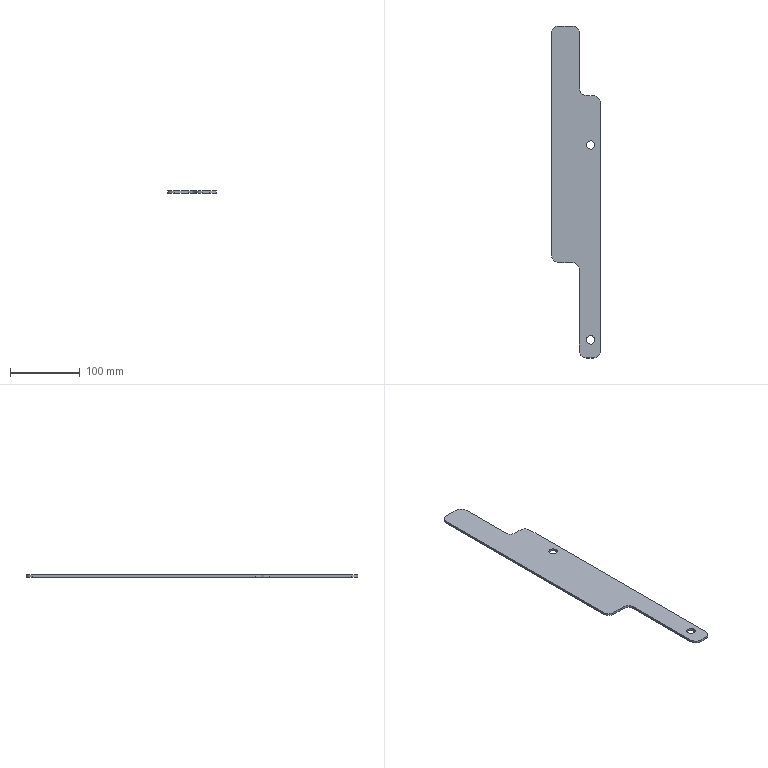Part | SolidWorks | features FlatPattern 1, SMBaseFlange 1, SheetMetal 1 | 1 solid | 22 faces | box 70 x 477 x 3.2 mm | volume 78713 mm3 | cylinder 12 | plane 10 | commonest cylinder face diameters 20 x8 12 x4
STEP:
#1=CARTESIAN_POINT('',(50.,-451.,-3.2));
#2=VERTEX_POINT('',#1);
#3=CARTESIAN_POINT('',(62.,-451.,-3.2));
#4=VERTEX_POINT('',#3);
#5=CARTESIAN_POINT('',(56.,-451.,-3.2));
#6=DIRECTION('',(0.,0.,1.));
#7=DIRECTION('',(1.,0.,0.));
#8=AXIS2_PLACEMENT_3D('',#5,#6,#7);
#9=CIRCLE('',#8,6.);
#10=EDGE_CURVE('',#2,#4,#9,.T.);
#11=ORIENTED_EDGE('',*,*,#10,.F.);
#12=CARTESIAN_POINT('',(50.,-451.,0.));
#13=VERTEX_POINT('',#12);
#14=CARTESIAN_POINT('',(50.,-451.,-3.2));
#15=DIRECTION('',(0.,0.,1.));
#16=VECTOR('',#15,1000.);
#17=LINE('',#14,#16);
#18=EDGE_CURVE('',#2,#13,#17,.T.);
#19=ORIENTED_EDGE('',*,*,#18,.T.);
#20=CARTESIAN_POINT('',(62.,-451.,0.));
#21=VERTEX_POINT('',#20);
#22=CARTESIAN_POINT('',(56.,-451.,0.));
#23=DIRECTION('',(0.,0.,1.));
#24=DIRECTION('',(1.,0.,0.));
#25=AXIS2_PLACEMENT_3D('',#22,#23,#24);
#26=CIRCLE('',#25,6.);
#27=EDGE_CURVE('',#13,#21,#26,.T.);
#28=ORIENTED_EDGE('',*,*,#27,.T.);
#29=CARTESIAN_POINT('',(62.,-451.,-3.2));
#30=DIRECTION('',(0.,0.,1.));
#31=VECTOR('',#30,1000.);
#32=LINE('',#29,#31);
#33=EDGE_CURVE('',#4,#21,#32,.T.);
#34=ORIENTED_EDGE('',*,*,#33,.F.);
#35=EDGE_LOOP('',(#11,#19,#28,#34));
#36=FACE_OUTER_BOUND('',#35,.T.);
#37=CARTESIAN_POINT('',(56.,-451.,-3.2));
#38=DIRECTION('',(0.,0.,1.));
#39=DIRECTION('',(1.,0.,0.));
#40=AXIS2_PLACEMENT_3D('',#37,#38,#39);
#41=CYLINDRICAL_SURFACE('',#40,6.);
#42=ADVANCED_FACE('',(#36),#41,.F.);
#43=CARTESIAN_POINT('',(50.,-171.,-3.2));
#44=VERTEX_POINT('',#43);
#45=CARTESIAN_POINT('',(62.,-171.,-3.2));
#46=VERTEX_POINT('',#45);
#47=CARTESIAN_POINT('',(56.,-171.,-3.2));
#48=DIRECTION('',(0.,0.,1.));
#49=DIRECTION('',(1.,0.,0.));
#50=AXIS2_PLACEMENT_3D('',#47,#48,#49);
#51=CIRCLE('',#50,6.);
#52=EDGE_CURVE('',#44,#46,#51,.T.);
#53=ORIENTED_EDGE('',*,*,#52,.F.);
#54=CARTESIAN_POINT('',(50.,-171.,0.));
#55=VERTEX_POINT('',#54);
#56=CARTESIAN_POINT('',(50.,-171.,-3.2));
#57=DIRECTION('',(0.,0.,1.));
#58=VECTOR('',#57,1000.);
#59=LINE('',#56,#58);
#60=EDGE_CURVE('',#44,#55,#59,.T.);
#61=ORIENTED_EDGE('',*,*,#60,.T.);
#62=CARTESIAN_POINT('',(62.,-171.,0.));
#63=VERTEX_POINT('',#62);
#64=CARTESIAN_POINT('',(56.,-171.,0.));
#65=DIRECTION('',(0.,0.,1.));
#66=DIRECTION('',(1.,0.,0.));
#67=AXIS2_PLACEMENT_3D('',#64,#65,#66);
#68=CIRCLE('',#67,6.);
#69=EDGE_CURVE('',#55,#63,#68,.T.);
#70=ORIENTED_EDGE('',*,*,#69,.T.);
#71=CARTESIAN_POINT('',(62.,-171.,-3.2));
#72=DIRECTION('',(0.,0.,1.));
#73=VECTOR('',#72,1000.);
#74=LINE('',#71,#73);
#75=EDGE_CURVE('',#46,#63,#74,.T.);
#76=ORIENTED_EDGE('',*,*,#75,.F.);
#77=EDGE_LOOP('',(#53,#61,#70,#76));
#78=FACE_OUTER_BOUND('',#77,.T.);
#79=CARTESIAN_POINT('',(56.,-171.,-3.2));
#80=DIRECTION('',(0.,0.,1.));
#81=DIRECTION('',(1.,0.,0.));
#82=AXIS2_PLACEMENT_3D('',#79,#80,#81);
#83=CYLINDRICAL_SURFACE('',#82,6.);
#84=ADVANCED_FACE('',(#78),#83,.F.);
#85=CARTESIAN_POINT('',(0.,-330.,0.));
#86=VERTEX_POINT('',#85);
#87=CARTESIAN_POINT('',(10.,-340.,0.));
#88=VERTEX_POINT('',#87);
#89=CARTESIAN_POINT('',(10.,-330.,0.));
#90=DIRECTION('',(0.,0.,1.));
#91=DIRECTION('',(-1.,0.,0.));
#92=AXIS2_PLACEMENT_3D('',#89,#90,#91);
#93=CIRCLE('',#92,10.);
#94=EDGE_CURVE('',#86,#88,#93,.T.);
#95=ORIENTED_EDGE('',*,*,#94,.F.);
#96=CARTESIAN_POINT('',(0.,-330.,-3.2));
#97=VERTEX_POINT('',#96);
#98=CARTESIAN_POINT('',(0.,-330.,-3.2));
#99=DIRECTION('',(0.,0.,1.));
#100=VECTOR('',#99,1000.);
#101=LINE('',#98,#100);
#102=EDGE_CURVE('',#97,#86,#101,.T.);
#103=ORIENTED_EDGE('',*,*,#102,.F.);
#104=CARTESIAN_POINT('',(10.,-340.,-3.2));
#105=VERTEX_POINT('',#104);
#106=CARTESIAN_POINT('',(10.,-330.,-3.2));
#107=DIRECTION('',(0.,0.,1.));
#108=DIRECTION('',(-1.,0.,0.));
#109=AXIS2_PLACEMENT_3D('',#106,#107,#108);
#110=CIRCLE('',#109,10.);
#111=EDGE_CURVE('',#97,#105,#110,.T.);
#112=ORIENTED_EDGE('',*,*,#111,.T.);
#113=CARTESIAN_POINT('',(10.,-340.,-3.2));
#114=DIRECTION('',(0.,0.,1.));
#115=VECTOR('',#114,1000.);
#116=LINE('',#113,#115);
#117=EDGE_CURVE('',#105,#88,#116,.T.);
#118=ORIENTED_EDGE('',*,*,#117,.T.);
#119=EDGE_LOOP('',(#95,#103,#112,#118));
#120=FACE_OUTER_BOUND('',#119,.T.);
#121=CARTESIAN_POINT('',(10.,-330.,-3.2));
#122=DIRECTION('',(0.,0.,1.));
#123=DIRECTION('',(1.,0.,0.));
#124=AXIS2_PLACEMENT_3D('',#121,#122,#123);
#125=CYLINDRICAL_SURFACE('',#124,10.);
#126=ADVANCED_FACE('',(#120),#125,.T.);
#127=CARTESIAN_POINT('',(0.,-10.,0.));
#128=VERTEX_POINT('',#127);
#129=CARTESIAN_POINT('',(0.,-330.,0.));
#130=DIRECTION('',(0.,-1.,0.));
#131=VECTOR('',#130,1000.);
#132=LINE('',#129,#131);
#133=EDGE_CURVE('',#128,#86,#132,.T.);
#134=ORIENTED_EDGE('',*,*,#133,.F.);
#135=CARTESIAN_POINT('',(0.,-10.,-3.2));
#136=VERTEX_POINT('',#135);
#137=CARTESIAN_POINT('',(0.,-10.,-3.2));
#138=DIRECTION('',(0.,0.,1.));
#139=VECTOR('',#138,1000.);
#140=LINE('',#137,#139);
#141=EDGE_CURVE('',#136,#128,#140,.T.);
#142=ORIENTED_EDGE('',*,*,#141,.F.);
#143=CARTESIAN_POINT('',(0.,-330.,-3.2));
#144=DIRECTION('',(0.,-1.,0.));
#145=VECTOR('',#144,1000.);
#146=LINE('',#143,#145);
#147=EDGE_CURVE('',#136,#97,#146,.T.);
#148=ORIENTED_EDGE('',*,*,#147,.T.);
#149=ORIENTED_EDGE('',*,*,#102,.T.);
#150=EDGE_LOOP('',(#134,#142,#148,#149));
#151=FACE_OUTER_BOUND('',#150,.T.);
#152=CARTESIAN_POINT('',(0.,-330.,-3.2));
#153=DIRECTION('',(-1.,0.,0.));
#154=DIRECTION('',(0.,0.,1.));
#155=AXIS2_PLACEMENT_3D('',#152,#153,#154);
#156=PLANE('',#155);
#157=ADVANCED_FACE('',(#151),#156,.T.);
#158=CARTESIAN_POINT('',(10.,0.,0.));
#159=VERTEX_POINT('',#158);
#160=CARTESIAN_POINT('',(10.,-10.,0.));
#161=DIRECTION('',(0.,0.,1.));
#162=DIRECTION('',(1.,0.,0.));
#163=AXIS2_PLACEMENT_3D('',#160,#161,#162);
#164=CIRCLE('',#163,10.);
#165=EDGE_CURVE('',#159,#128,#164,.T.);
#166=ORIENTED_EDGE('',*,*,#165,.F.);
#167=CARTESIAN_POINT('',(10.,0.,-3.2));
#168=VERTEX_POINT('',#167);
#169=CARTESIAN_POINT('',(10.,0.,-3.2));
#170=DIRECTION('',(0.,0.,1.));
#171=VECTOR('',#170,1000.);
#172=LINE('',#169,#171);
#173=EDGE_CURVE('',#168,#159,#172,.T.);
#174=ORIENTED_EDGE('',*,*,#173,.F.);
#175=CARTESIAN_POINT('',(10.,-10.,-3.2));
#176=DIRECTION('',(0.,0.,1.));
#177=DIRECTION('',(1.,0.,0.));
#178=AXIS2_PLACEMENT_3D('',#175,#176,#177);
#179=CIRCLE('',#178,10.);
#180=EDGE_CURVE('',#168,#136,#179,.T.);
#181=ORIENTED_EDGE('',*,*,#180,.T.);
#182=ORIENTED_EDGE('',*,*,#141,.T.);
#183=EDGE_LOOP('',(#166,#174,#181,#182));
#184=FACE_OUTER_BOUND('',#183,.T.);
#185=CARTESIAN_POINT('',(10.,-10.,-3.2));
#186=DIRECTION('',(0.,0.,1.));
#187=DIRECTION('',(1.,0.,0.));
#188=AXIS2_PLACEMENT_3D('',#185,#186,#187);
#189=CYLINDRICAL_SURFACE('',#188,10.);
#190=ADVANCED_FACE('',(#184),#189,.T.);
#191=CARTESIAN_POINT('',(30.,0.,0.));
#192=VERTEX_POINT('',#191);
#193=CARTESIAN_POINT('',(10.,0.,0.));
#194=DIRECTION('',(-1.,0.,0.));
#195=VECTOR('',#194,1000.);
#196=LINE('',#193,#195);
#197=EDGE_CURVE('',#192,#159,#196,.T.);
#198=ORIENTED_EDGE('',*,*,#197,.F.);
#199=CARTESIAN_POINT('',(30.,0.,-3.2));
#200=VERTEX_POINT('',#199);
#201=CARTESIAN_POINT('',(30.,0.,-3.2));
#202=DIRECTION('',(0.,0.,1.));
#203=VECTOR('',#202,1000.);
#204=LINE('',#201,#203);
#205=EDGE_CURVE('',#200,#192,#204,.T.);
#206=ORIENTED_EDGE('',*,*,#205,.F.);
#207=CARTESIAN_POINT('',(10.,0.,-3.2));
#208=DIRECTION('',(-1.,0.,0.));
#209=VECTOR('',#208,1000.);
#210=LINE('',#207,#209);
#211=EDGE_CURVE('',#200,#168,#210,.T.);
#212=ORIENTED_EDGE('',*,*,#211,.T.);
#213=ORIENTED_EDGE('',*,*,#173,.T.);
#214=EDGE_LOOP('',(#198,#206,#212,#213));
#215=FACE_OUTER_BOUND('',#214,.T.);
#216=CARTESIAN_POINT('',(10.,0.,-3.2));
#217=DIRECTION('',(0.,1.,0.));
#218=DIRECTION('',(0.,0.,1.));
#219=AXIS2_PLACEMENT_3D('',#216,#217,#218);
#220=PLANE('',#219);
#221=ADVANCED_FACE('',(#215),#220,.T.);
#222=CARTESIAN_POINT('',(40.,-10.,0.));
#223=VERTEX_POINT('',#222);
#224=CARTESIAN_POINT('',(30.,-10.,0.));
#225=DIRECTION('',(0.,0.,1.));
#226=DIRECTION('',(-1.,0.,0.));
#227=AXIS2_PLACEMENT_3D('',#224,#225,#226);
#228=CIRCLE('',#227,10.);
#229=EDGE_CURVE('',#223,#192,#228,.T.);
#230=ORIENTED_EDGE('',*,*,#229,.F.);
#231=CARTESIAN_POINT('',(40.,-10.,-3.2));
#232=VERTEX_POINT('',#231);
#233=CARTESIAN_POINT('',(40.,-10.,-3.2));
#234=DIRECTION('',(0.,0.,1.));
#235=VECTOR('',#234,1000.);
#236=LINE('',#233,#235);
#237=EDGE_CURVE('',#232,#223,#236,.T.);
#238=ORIENTED_EDGE('',*,*,#237,.F.);
#239=CARTESIAN_POINT('',(30.,-10.,-3.2));
#240=DIRECTION('',(0.,0.,1.));
#241=DIRECTION('',(-1.,0.,0.));
#242=AXIS2_PLACEMENT_3D('',#239,#240,#241);
#243=CIRCLE('',#242,10.);
#244=EDGE_CURVE('',#232,#200,#243,.T.);
#245=ORIENTED_EDGE('',*,*,#244,.T.);
#246=ORIENTED_EDGE('',*,*,#205,.T.);
#247=EDGE_LOOP('',(#230,#238,#245,#246));
#248=FACE_OUTER_BOUND('',#247,.T.);
#249=CARTESIAN_POINT('',(30.,-10.,-3.2));
#250=DIRECTION('',(0.,0.,1.));
#251=DIRECTION('',(1.,0.,0.));
#252=AXIS2_PLACEMENT_3D('',#249,#250,#251);
#253=CYLINDRICAL_SURFACE('',#252,10.);
#254=ADVANCED_FACE('',(#248),#253,.T.);
#255=CARTESIAN_POINT('',(40.,-90.,0.));
#256=VERTEX_POINT('',#255);
#257=CARTESIAN_POINT('',(40.,-10.,0.));
#258=DIRECTION('',(0.,1.,0.));
#259=VECTOR('',#258,1000.);
#260=LINE('',#257,#259);
#261=EDGE_CURVE('',#256,#223,#260,.T.);
#262=ORIENTED_EDGE('',*,*,#261,.F.);
#263=CARTESIAN_POINT('',(40.,-90.,-3.2));
#264=VERTEX_POINT('',#263);
#265=CARTESIAN_POINT('',(40.,-90.,-3.2));
#266=DIRECTION('',(0.,0.,1.));
#267=VECTOR('',#266,1000.);
#268=LINE('',#265,#267);
#269=EDGE_CURVE('',#264,#256,#268,.T.);
#270=ORIENTED_EDGE('',*,*,#269,.F.);
#271=CARTESIAN_POINT('',(40.,-10.,-3.2));
#272=DIRECTION('',(0.,1.,0.));
#273=VECTOR('',#272,1000.);
#274=LINE('',#271,#273);
#275=EDGE_CURVE('',#264,#232,#274,.T.);
#276=ORIENTED_EDGE('',*,*,#275,.T.);
#277=ORIENTED_EDGE('',*,*,#237,.T.);
#278=EDGE_LOOP('',(#262,#270,#276,#277));
#279=FACE_OUTER_BOUND('',#278,.T.);
#280=CARTESIAN_POINT('',(40.,-10.,-3.2));
#281=DIRECTION('',(1.,0.,0.));
#282=DIRECTION('',(0.,1.,0.));
#283=AXIS2_PLACEMENT_3D('',#280,#281,#282);
#284=PLANE('',#283);
#285=ADVANCED_FACE('',(#279),#284,.T.);
#286=CARTESIAN_POINT('',(50.,-100.,0.));
#287=VERTEX_POINT('',#286);
#288=CARTESIAN_POINT('',(50.,-90.,0.));
#289=DIRECTION('',(0.,0.,-1.));
#290=DIRECTION('',(1.,0.,0.));
#291=AXIS2_PLACEMENT_3D('',#288,#289,#290);
#292=CIRCLE('',#291,10.);
#293=EDGE_CURVE('',#287,#256,#292,.T.);
#294=ORIENTED_EDGE('',*,*,#293,.F.);
#295=CARTESIAN_POINT('',(50.,-100.,-3.2));
#296=VERTEX_POINT('',#295);
#297=CARTESIAN_POINT('',(50.,-100.,-3.2));
#298=DIRECTION('',(0.,0.,1.));
#299=VECTOR('',#298,1000.);
#300=LINE('',#297,#299);
#301=EDGE_CURVE('',#296,#287,#300,.T.);
#302=ORIENTED_EDGE('',*,*,#301,.F.);
#303=CARTESIAN_POINT('',(50.,-90.,-3.2));
#304=DIRECTION('',(0.,0.,-1.));
#305=DIRECTION('',(1.,0.,0.));
#306=AXIS2_PLACEMENT_3D('',#303,#304,#305);
#307=CIRCLE('',#306,10.);
#308=EDGE_CURVE('',#296,#264,#307,.T.);
#309=ORIENTED_EDGE('',*,*,#308,.T.);
#310=ORIENTED_EDGE('',*,*,#269,.T.);
#311=EDGE_LOOP('',(#294,#302,#309,#310));
#312=FACE_OUTER_BOUND('',#311,.T.);
#313=CARTESIAN_POINT('',(50.,-90.,-3.2));
#314=DIRECTION('',(0.,0.,1.));
#315=DIRECTION('',(1.,0.,0.));
#316=AXIS2_PLACEMENT_3D('',#313,#314,#315);
#317=CYLINDRICAL_SURFACE('',#316,10.);
#318=ADVANCED_FACE('',(#312),#317,.F.);
#319=CARTESIAN_POINT('',(60.,-100.,0.));
#320=VERTEX_POINT('',#319);
#321=CARTESIAN_POINT('',(50.,-100.,0.));
#322=DIRECTION('',(-1.,0.,0.));
#323=VECTOR('',#322,1000.);
#324=LINE('',#321,#323);
#325=EDGE_CURVE('',#320,#287,#324,.T.);
#326=ORIENTED_EDGE('',*,*,#325,.F.);
#327=CARTESIAN_POINT('',(60.,-100.,-3.2));
#328=VERTEX_POINT('',#327);
#329=CARTESIAN_POINT('',(60.,-100.,-3.2));
#330=DIRECTION('',(0.,0.,1.));
#331=VECTOR('',#330,1000.);
#332=LINE('',#329,#331);
#333=EDGE_CURVE('',#328,#320,#332,.T.);
#334=ORIENTED_EDGE('',*,*,#333,.F.);
#335=CARTESIAN_POINT('',(50.,-100.,-3.2));
#336=DIRECTION('',(-1.,0.,0.));
#337=VECTOR('',#336,1000.);
#338=LINE('',#335,#337);
#339=EDGE_CURVE('',#328,#296,#338,.T.);
#340=ORIENTED_EDGE('',*,*,#339,.T.);
#341=ORIENTED_EDGE('',*,*,#301,.T.);
#342=EDGE_LOOP('',(#326,#334,#340,#341));
#343=FACE_OUTER_BOUND('',#342,.T.);
#344=CARTESIAN_POINT('',(50.,-100.,-3.2));
#345=DIRECTION('',(0.,1.,0.));
#346=DIRECTION('',(0.,0.,1.));
#347=AXIS2_PLACEMENT_3D('',#344,#345,#346);
#348=PLANE('',#347);
#349=ADVANCED_FACE('',(#343),#348,.T.);
#350=CARTESIAN_POINT('',(70.,-110.,0.));
#351=VERTEX_POINT('',#350);
#352=CARTESIAN_POINT('',(60.,-110.,0.));
#353=DIRECTION('',(0.,0.,1.));
#354=DIRECTION('',(-1.,0.,0.));
#355=AXIS2_PLACEMENT_3D('',#352,#353,#354);
#356=CIRCLE('',#355,10.);
#357=EDGE_CURVE('',#351,#320,#356,.T.);
#358=ORIENTED_EDGE('',*,*,#357,.F.);
#359=CARTESIAN_POINT('',(70.,-110.,-3.2));
#360=VERTEX_POINT('',#359);
#361=CARTESIAN_POINT('',(70.,-110.,-3.2));
#362=DIRECTION('',(0.,0.,1.));
#363=VECTOR('',#362,1000.);
#364=LINE('',#361,#363);
#365=EDGE_CURVE('',#360,#351,#364,.T.);
#366=ORIENTED_EDGE('',*,*,#365,.F.);
#367=CARTESIAN_POINT('',(60.,-110.,-3.2));
#368=DIRECTION('',(0.,0.,1.));
#369=DIRECTION('',(-1.,0.,0.));
#370=AXIS2_PLACEMENT_3D('',#367,#368,#369);
#371=CIRCLE('',#370,10.);
#372=EDGE_CURVE('',#360,#328,#371,.T.);
#373=ORIENTED_EDGE('',*,*,#372,.T.);
#374=ORIENTED_EDGE('',*,*,#333,.T.);
#375=EDGE_LOOP('',(#358,#366,#373,#374));
#376=FACE_OUTER_BOUND('',#375,.T.);
#377=CARTESIAN_POINT('',(60.,-110.,-3.2));
#378=DIRECTION('',(0.,0.,1.));
#379=DIRECTION('',(1.,0.,0.));
#380=AXIS2_PLACEMENT_3D('',#377,#378,#379);
#381=CYLINDRICAL_SURFACE('',#380,10.);
#382=ADVANCED_FACE('',(#376),#381,.T.);
#383=CARTESIAN_POINT('',(70.,-467.,0.));
#384=VERTEX_POINT('',#383);
#385=CARTESIAN_POINT('',(70.,-110.,0.));
#386=DIRECTION('',(0.,1.,0.));
#387=VECTOR('',#386,1000.);
#388=LINE('',#385,#387);
#389=EDGE_CURVE('',#384,#351,#388,.T.);
#390=ORIENTED_EDGE('',*,*,#389,.F.);
#391=CARTESIAN_POINT('',(70.,-467.,-3.2));
#392=VERTEX_POINT('',#391);
#393=CARTESIAN_POINT('',(70.,-467.,-3.2));
#394=DIRECTION('',(0.,0.,1.));
#395=VECTOR('',#394,1000.);
#396=LINE('',#393,#395);
#397=EDGE_CURVE('',#392,#384,#396,.T.);
#398=ORIENTED_EDGE('',*,*,#397,.F.);
#399=CARTESIAN_POINT('',(70.,-110.,-3.2));
#400=DIRECTION('',(0.,1.,0.));
#401=VECTOR('',#400,1000.);
#402=LINE('',#399,#401);
#403=EDGE_CURVE('',#392,#360,#402,.T.);
#404=ORIENTED_EDGE('',*,*,#403,.T.);
#405=ORIENTED_EDGE('',*,*,#365,.T.);
#406=EDGE_LOOP('',(#390,#398,#404,#405));
#407=FACE_OUTER_BOUND('',#406,.T.);
#408=CARTESIAN_POINT('',(70.,-110.,-3.2));
#409=DIRECTION('',(1.,0.,0.));
#410=DIRECTION('',(0.,1.,0.));
#411=AXIS2_PLACEMENT_3D('',#408,#409,#410);
#412=PLANE('',#411);
#413=ADVANCED_FACE('',(#407),#412,.T.);
#414=CARTESIAN_POINT('',(60.,-477.,0.));
#415=VERTEX_POINT('',#414);
#416=CARTESIAN_POINT('',(60.,-467.,0.));
#417=DIRECTION('',(0.,0.,1.));
#418=DIRECTION('',(-1.,0.,0.));
#419=AXIS2_PLACEMENT_3D('',#416,#417,#418);
#420=CIRCLE('',#419,10.);
#421=EDGE_CURVE('',#415,#384,#420,.T.);
#422=ORIENTED_EDGE('',*,*,#421,.F.);
#423=CARTESIAN_POINT('',(60.,-477.,-3.2));
#424=VERTEX_POINT('',#423);
#425=CARTESIAN_POINT('',(60.,-477.,-3.2));
#426=DIRECTION('',(0.,0.,1.));
#427=VECTOR('',#426,1000.);
#428=LINE('',#425,#427);
#429=EDGE_CURVE('',#424,#415,#428,.T.);
#430=ORIENTED_EDGE('',*,*,#429,.F.);
#431=CARTESIAN_POINT('',(60.,-467.,-3.2));
#432=DIRECTION('',(0.,0.,1.));
#433=DIRECTION('',(-1.,0.,0.));
#434=AXIS2_PLACEMENT_3D('',#431,#432,#433);
#435=CIRCLE('',#434,10.);
#436=EDGE_CURVE('',#424,#392,#435,.T.);
#437=ORIENTED_EDGE('',*,*,#436,.T.);
#438=ORIENTED_EDGE('',*,*,#397,.T.);
#439=EDGE_LOOP('',(#422,#430,#437,#438));
#440=FACE_OUTER_BOUND('',#439,.T.);
#441=CARTESIAN_POINT('',(60.,-467.,-3.2));
#442=DIRECTION('',(0.,0.,1.));
#443=DIRECTION('',(1.,0.,0.));
#444=AXIS2_PLACEMENT_3D('',#441,#442,#443);
#445=CYLINDRICAL_SURFACE('',#444,10.);
#446=ADVANCED_FACE('',(#440),#445,.T.);
#447=CARTESIAN_POINT('',(50.,-477.,0.));
#448=VERTEX_POINT('',#447);
#449=CARTESIAN_POINT('',(60.,-477.,0.));
#450=DIRECTION('',(1.,0.,0.));
#451=VECTOR('',#450,1000.);
#452=LINE('',#449,#451);
#453=EDGE_CURVE('',#448,#415,#452,.T.);
#454=ORIENTED_EDGE('',*,*,#453,.F.);
#455=CARTESIAN_POINT('',(50.,-477.,-3.2));
#456=VERTEX_POINT('',#455);
#457=CARTESIAN_POINT('',(50.,-477.,-3.2));
#458=DIRECTION('',(0.,0.,1.));
#459=VECTOR('',#458,1000.);
#460=LINE('',#457,#459);
#461=EDGE_CURVE('',#456,#448,#460,.T.);
#462=ORIENTED_EDGE('',*,*,#461,.F.);
#463=CARTESIAN_POINT('',(60.,-477.,-3.2));
#464=DIRECTION('',(1.,0.,0.));
#465=VECTOR('',#464,1000.);
#466=LINE('',#463,#465);
#467=EDGE_CURVE('',#456,#424,#466,.T.);
#468=ORIENTED_EDGE('',*,*,#467,.T.);
#469=ORIENTED_EDGE('',*,*,#429,.T.);
#470=EDGE_LOOP('',(#454,#462,#468,#469));
#471=FACE_OUTER_BOUND('',#470,.T.);
#472=CARTESIAN_POINT('',(60.,-477.,-3.2));
#473=DIRECTION('',(0.,-1.,0.));
#474=DIRECTION('',(0.,0.,-1.));
#475=AXIS2_PLACEMENT_3D('',#472,#473,#474);
#476=PLANE('',#475);
#477=ADVANCED_FACE('',(#471),#476,.T.);
#478=CARTESIAN_POINT('',(40.,-467.,0.));
#479=VERTEX_POINT('',#478);
#480=CARTESIAN_POINT('',(50.,-467.,0.));
#481=DIRECTION('',(0.,0.,1.));
#482=DIRECTION('',(-1.,0.,0.));
#483=AXIS2_PLACEMENT_3D('',#480,#481,#482);
#484=CIRCLE('',#483,10.);
#485=EDGE_CURVE('',#479,#448,#484,.T.);
#486=ORIENTED_EDGE('',*,*,#485,.F.);
#487=CARTESIAN_POINT('',(40.,-467.,-3.2));
#488=VERTEX_POINT('',#487);
#489=CARTESIAN_POINT('',(40.,-467.,-3.2));
#490=DIRECTION('',(0.,0.,1.));
#491=VECTOR('',#490,1000.);
#492=LINE('',#489,#491);
#493=EDGE_CURVE('',#488,#479,#492,.T.);
#494=ORIENTED_EDGE('',*,*,#493,.F.);
#495=CARTESIAN_POINT('',(50.,-467.,-3.2));
#496=DIRECTION('',(0.,0.,1.));
#497=DIRECTION('',(-1.,0.,0.));
#498=AXIS2_PLACEMENT_3D('',#495,#496,#497);
#499=CIRCLE('',#498,10.);
#500=EDGE_CURVE('',#488,#456,#499,.T.);
#501=ORIENTED_EDGE('',*,*,#500,.T.);
#502=ORIENTED_EDGE('',*,*,#461,.T.);
#503=EDGE_LOOP('',(#486,#494,#501,#502));
#504=FACE_OUTER_BOUND('',#503,.T.);
#505=CARTESIAN_POINT('',(50.,-467.,-3.2));
#506=DIRECTION('',(0.,0.,1.));
#507=DIRECTION('',(1.,0.,0.));
#508=AXIS2_PLACEMENT_3D('',#505,#506,#507);
#509=CYLINDRICAL_SURFACE('',#508,10.);
#510=ADVANCED_FACE('',(#504),#509,.T.);
#511=CARTESIAN_POINT('',(40.,-350.,0.));
#512=VERTEX_POINT('',#511);
#513=CARTESIAN_POINT('',(40.,-467.,0.));
#514=DIRECTION('',(0.,-1.,0.));
#515=VECTOR('',#514,1000.);
#516=LINE('',#513,#515);
#517=EDGE_CURVE('',#512,#479,#516,.T.);
#518=ORIENTED_EDGE('',*,*,#517,.F.);
#519=CARTESIAN_POINT('',(40.,-350.,-3.2));
#520=VERTEX_POINT('',#519);
#521=CARTESIAN_POINT('',(40.,-350.,-3.2));
#522=DIRECTION('',(0.,0.,1.));
#523=VECTOR('',#522,1000.);
#524=LINE('',#521,#523);
#525=EDGE_CURVE('',#520,#512,#524,.T.);
#526=ORIENTED_EDGE('',*,*,#525,.F.);
#527=CARTESIAN_POINT('',(40.,-467.,-3.2));
#528=DIRECTION('',(0.,-1.,0.));
#529=VECTOR('',#528,1000.);
#530=LINE('',#527,#529);
#531=EDGE_CURVE('',#520,#488,#530,.T.);
#532=ORIENTED_EDGE('',*,*,#531,.T.);
#533=ORIENTED_EDGE('',*,*,#493,.T.);
#534=EDGE_LOOP('',(#518,#526,#532,#533));
#535=FACE_OUTER_BOUND('',#534,.T.);
#536=CARTESIAN_POINT('',(40.,-467.,-3.2));
#537=DIRECTION('',(-1.,0.,0.));
#538=DIRECTION('',(0.,0.,1.));
#539=AXIS2_PLACEMENT_3D('',#536,#537,#538);
#540=PLANE('',#539);
#541=ADVANCED_FACE('',(#535),#540,.T.);
#542=CARTESIAN_POINT('',(30.,-340.,0.));
#543=VERTEX_POINT('',#542);
#544=CARTESIAN_POINT('',(30.,-350.,0.));
#545=DIRECTION('',(0.,0.,-1.));
#546=DIRECTION('',(1.,0.,0.));
#547=AXIS2_PLACEMENT_3D('',#544,#545,#546);
#548=CIRCLE('',#547,10.);
#549=EDGE_CURVE('',#543,#512,#548,.T.);
#550=ORIENTED_EDGE('',*,*,#549,.F.);
#551=CARTESIAN_POINT('',(30.,-340.,-3.2));
#552=VERTEX_POINT('',#551);
#553=CARTESIAN_POINT('',(30.,-340.,-3.2));
#554=DIRECTION('',(0.,0.,1.));
#555=VECTOR('',#554,1000.);
#556=LINE('',#553,#555);
#557=EDGE_CURVE('',#552,#543,#556,.T.);
#558=ORIENTED_EDGE('',*,*,#557,.F.);
#559=CARTESIAN_POINT('',(30.,-350.,-3.2));
#560=DIRECTION('',(0.,0.,-1.));
#561=DIRECTION('',(1.,0.,0.));
#562=AXIS2_PLACEMENT_3D('',#559,#560,#561);
#563=CIRCLE('',#562,10.);
#564=EDGE_CURVE('',#552,#520,#563,.T.);
#565=ORIENTED_EDGE('',*,*,#564,.T.);
#566=ORIENTED_EDGE('',*,*,#525,.T.);
#567=EDGE_LOOP('',(#550,#558,#565,#566));
#568=FACE_OUTER_BOUND('',#567,.T.);
#569=CARTESIAN_POINT('',(30.,-350.,-3.2));
#570=DIRECTION('',(0.,0.,1.));
#571=DIRECTION('',(1.,0.,0.));
#572=AXIS2_PLACEMENT_3D('',#569,#570,#571);
#573=CYLINDRICAL_SURFACE('',#572,10.);
#574=ADVANCED_FACE('',(#568),#573,.F.);
#575=CARTESIAN_POINT('',(30.,-340.,0.));
#576=DIRECTION('',(1.,0.,0.));
#577=VECTOR('',#576,1000.);
#578=LINE('',#575,#577);
#579=EDGE_CURVE('',#88,#543,#578,.T.);
#580=ORIENTED_EDGE('',*,*,#579,.F.);
#581=ORIENTED_EDGE('',*,*,#117,.F.);
#582=CARTESIAN_POINT('',(30.,-340.,-3.2));
#583=DIRECTION('',(1.,0.,0.));
#584=VECTOR('',#583,1000.);
#585=LINE('',#582,#584);
#586=EDGE_CURVE('',#105,#552,#585,.T.);
#587=ORIENTED_EDGE('',*,*,#586,.T.);
#588=ORIENTED_EDGE('',*,*,#557,.T.);
#589=EDGE_LOOP('',(#580,#581,#587,#588));
#590=FACE_OUTER_BOUND('',#589,.T.);
#591=CARTESIAN_POINT('',(30.,-340.,-3.2));
#592=DIRECTION('',(0.,-1.,0.));
#593=DIRECTION('',(0.,0.,-1.));
#594=AXIS2_PLACEMENT_3D('',#591,#592,#593);
#595=PLANE('',#594);
#596=ADVANCED_FACE('',(#590),#595,.T.);
#597=CARTESIAN_POINT('',(56.,-451.,-3.2));
#598=DIRECTION('',(0.,0.,1.));
#599=DIRECTION('',(1.,0.,0.));
#600=AXIS2_PLACEMENT_3D('',#597,#598,#599);
#601=CIRCLE('',#600,6.);
#602=EDGE_CURVE('',#4,#2,#601,.T.);
#603=ORIENTED_EDGE('',*,*,#602,.T.);
#604=ORIENTED_EDGE('',*,*,#10,.T.);
#605=EDGE_LOOP('',(#603,#604));
#606=FACE_BOUND('',#605,.T.);
#607=CARTESIAN_POINT('',(56.,-171.,-3.2));
#608=DIRECTION('',(0.,0.,1.));
#609=DIRECTION('',(1.,0.,0.));
#610=AXIS2_PLACEMENT_3D('',#607,#608,#609);
#611=CIRCLE('',#610,6.);
#612=EDGE_CURVE('',#46,#44,#611,.T.);
#613=ORIENTED_EDGE('',*,*,#612,.T.);
#614=ORIENTED_EDGE('',*,*,#52,.T.);
#615=EDGE_LOOP('',(#613,#614));
#616=FACE_BOUND('',#615,.T.);
#617=ORIENTED_EDGE('',*,*,#111,.F.);
#618=ORIENTED_EDGE('',*,*,#147,.F.);
#619=ORIENTED_EDGE('',*,*,#180,.F.);
#620=ORIENTED_EDGE('',*,*,#211,.F.);
#621=ORIENTED_EDGE('',*,*,#244,.F.);
#622=ORIENTED_EDGE('',*,*,#275,.F.);
#623=ORIENTED_EDGE('',*,*,#308,.F.);
#624=ORIENTED_EDGE('',*,*,#339,.F.);
#625=ORIENTED_EDGE('',*,*,#372,.F.);
#626=ORIENTED_EDGE('',*,*,#403,.F.);
#627=ORIENTED_EDGE('',*,*,#436,.F.);
#628=ORIENTED_EDGE('',*,*,#467,.F.);
#629=ORIENTED_EDGE('',*,*,#500,.F.);
#630=ORIENTED_EDGE('',*,*,#531,.F.);
#631=ORIENTED_EDGE('',*,*,#564,.F.);
#632=ORIENTED_EDGE('',*,*,#586,.F.);
#633=EDGE_LOOP('',(#617,#618,#619,#620,#621,#622,#623,#624,#625,#626,#627,#628,#629,#630,#631,#632));
#634=FACE_OUTER_BOUND('',#633,.T.);
#635=CARTESIAN_POINT('',(10.,-330.,-3.2));
#636=DIRECTION('',(0.,0.,-1.));
#637=DIRECTION('',(-1.,0.,0.));
#638=AXIS2_PLACEMENT_3D('',#635,#636,#637);
#639=PLANE('',#638);
#640=ADVANCED_FACE('',(#606,#616,#634),#639,.T.);
#641=CARTESIAN_POINT('',(56.,-451.,0.));
#642=DIRECTION('',(0.,0.,1.));
#643=DIRECTION('',(1.,0.,0.));
#644=AXIS2_PLACEMENT_3D('',#641,#642,#643);
#645=CIRCLE('',#644,6.);
#646=EDGE_CURVE('',#21,#13,#645,.T.);
#647=ORIENTED_EDGE('',*,*,#646,.F.);
#648=ORIENTED_EDGE('',*,*,#27,.F.);
#649=EDGE_LOOP('',(#647,#648));
#650=FACE_BOUND('',#649,.T.);
#651=CARTESIAN_POINT('',(56.,-171.,0.));
#652=DIRECTION('',(0.,0.,1.));
#653=DIRECTION('',(1.,0.,0.));
#654=AXIS2_PLACEMENT_3D('',#651,#652,#653);
#655=CIRCLE('',#654,6.);
#656=EDGE_CURVE('',#63,#55,#655,.T.);
#657=ORIENTED_EDGE('',*,*,#656,.F.);
#658=ORIENTED_EDGE('',*,*,#69,.F.);
#659=EDGE_LOOP('',(#657,#658));
#660=FACE_BOUND('',#659,.T.);
#661=ORIENTED_EDGE('',*,*,#94,.T.);
#662=ORIENTED_EDGE('',*,*,#579,.T.);
#663=ORIENTED_EDGE('',*,*,#549,.T.);
#664=ORIENTED_EDGE('',*,*,#517,.T.);
#665=ORIENTED_EDGE('',*,*,#485,.T.);
#666=ORIENTED_EDGE('',*,*,#453,.T.);
#667=ORIENTED_EDGE('',*,*,#421,.T.);
#668=ORIENTED_EDGE('',*,*,#389,.T.);
#669=ORIENTED_EDGE('',*,*,#357,.T.);
#670=ORIENTED_EDGE('',*,*,#325,.T.);
#671=ORIENTED_EDGE('',*,*,#293,.T.);
#672=ORIENTED_EDGE('',*,*,#261,.T.);
#673=ORIENTED_EDGE('',*,*,#229,.T.);
#674=ORIENTED_EDGE('',*,*,#197,.T.);
#675=ORIENTED_EDGE('',*,*,#165,.T.);
#676=ORIENTED_EDGE('',*,*,#133,.T.);
#677=EDGE_LOOP('',(#661,#662,#663,#664,#665,#666,#667,#668,#669,#670,#671,#672,#673,#674,#675,#676));
#678=FACE_OUTER_BOUND('',#677,.T.);
#679=CARTESIAN_POINT('',(10.,-330.,0.));
#680=DIRECTION('',(0.,0.,-1.));
#681=DIRECTION('',(-1.,0.,0.));
#682=AXIS2_PLACEMENT_3D('',#679,#680,#681);
#683=PLANE('',#682);
#684=ADVANCED_FACE('',(#650,#660,#678),#683,.F.);
#685=ORIENTED_EDGE('',*,*,#60,.F.);
#686=ORIENTED_EDGE('',*,*,#612,.F.);
#687=ORIENTED_EDGE('',*,*,#75,.T.);
#688=ORIENTED_EDGE('',*,*,#656,.T.);
#689=EDGE_LOOP('',(#685,#686,#687,#688));
#690=FACE_OUTER_BOUND('',#689,.T.);
#691=CARTESIAN_POINT('',(56.,-171.,-3.2));
#692=DIRECTION('',(0.,0.,1.));
#693=DIRECTION('',(1.,0.,0.));
#694=AXIS2_PLACEMENT_3D('',#691,#692,#693);
#695=CYLINDRICAL_SURFACE('',#694,6.);
#696=ADVANCED_FACE('',(#690),#695,.F.);
#697=ORIENTED_EDGE('',*,*,#18,.F.);
#698=ORIENTED_EDGE('',*,*,#602,.F.);
#699=ORIENTED_EDGE('',*,*,#33,.T.);
#700=ORIENTED_EDGE('',*,*,#646,.T.);
#701=EDGE_LOOP('',(#697,#698,#699,#700));
#702=FACE_OUTER_BOUND('',#701,.T.);
#703=CARTESIAN_POINT('',(56.,-451.,-3.2));
#704=DIRECTION('',(0.,0.,1.));
#705=DIRECTION('',(1.,0.,0.));
#706=AXIS2_PLACEMENT_3D('',#703,#704,#705);
#707=CYLINDRICAL_SURFACE('',#706,6.);
#708=ADVANCED_FACE('',(#702),#707,.F.);
#709=CLOSED_SHELL('',(#42,#84,#126,#157,#190,#221,#254,#285,#318,#349,#382,#413,#446,#477,#510,#541,#574,#596,#640,#684,#696,#708));
#710=MANIFOLD_SOLID_BREP('',#709);
#711=CARTESIAN_POINT('',(0.,0.,0.));
#712=DIRECTION('',(0.,0.,1.));
#713=DIRECTION('',(1.,0.,0.));
#714=AXIS2_PLACEMENT_3D('',#711,#712,#713);
#715=(LENGTH_UNIT()NAMED_UNIT(*)SI_UNIT(.MILLI.,.METRE.));
#716=UNCERTAINTY_MEASURE_WITH_UNIT(LENGTH_MEASURE(0.00001),#715,'','');
#717=(NAMED_UNIT(*)PLANE_ANGLE_UNIT()SI_UNIT($,.RADIAN.));
#718=(NAMED_UNIT(*)SI_UNIT($,.STERADIAN.)SOLID_ANGLE_UNIT());
#719=(GEOMETRIC_REPRESENTATION_CONTEXT(3)GLOBAL_UNCERTAINTY_ASSIGNED_CONTEXT((#716))GLOBAL_UNIT_ASSIGNED_CONTEXT((#715,#717,#718))REPRESENTATION_CONTEXT('',''));
#720=ADVANCED_BREP_SHAPE_REPRESENTATION('',(#710,#714),#719);